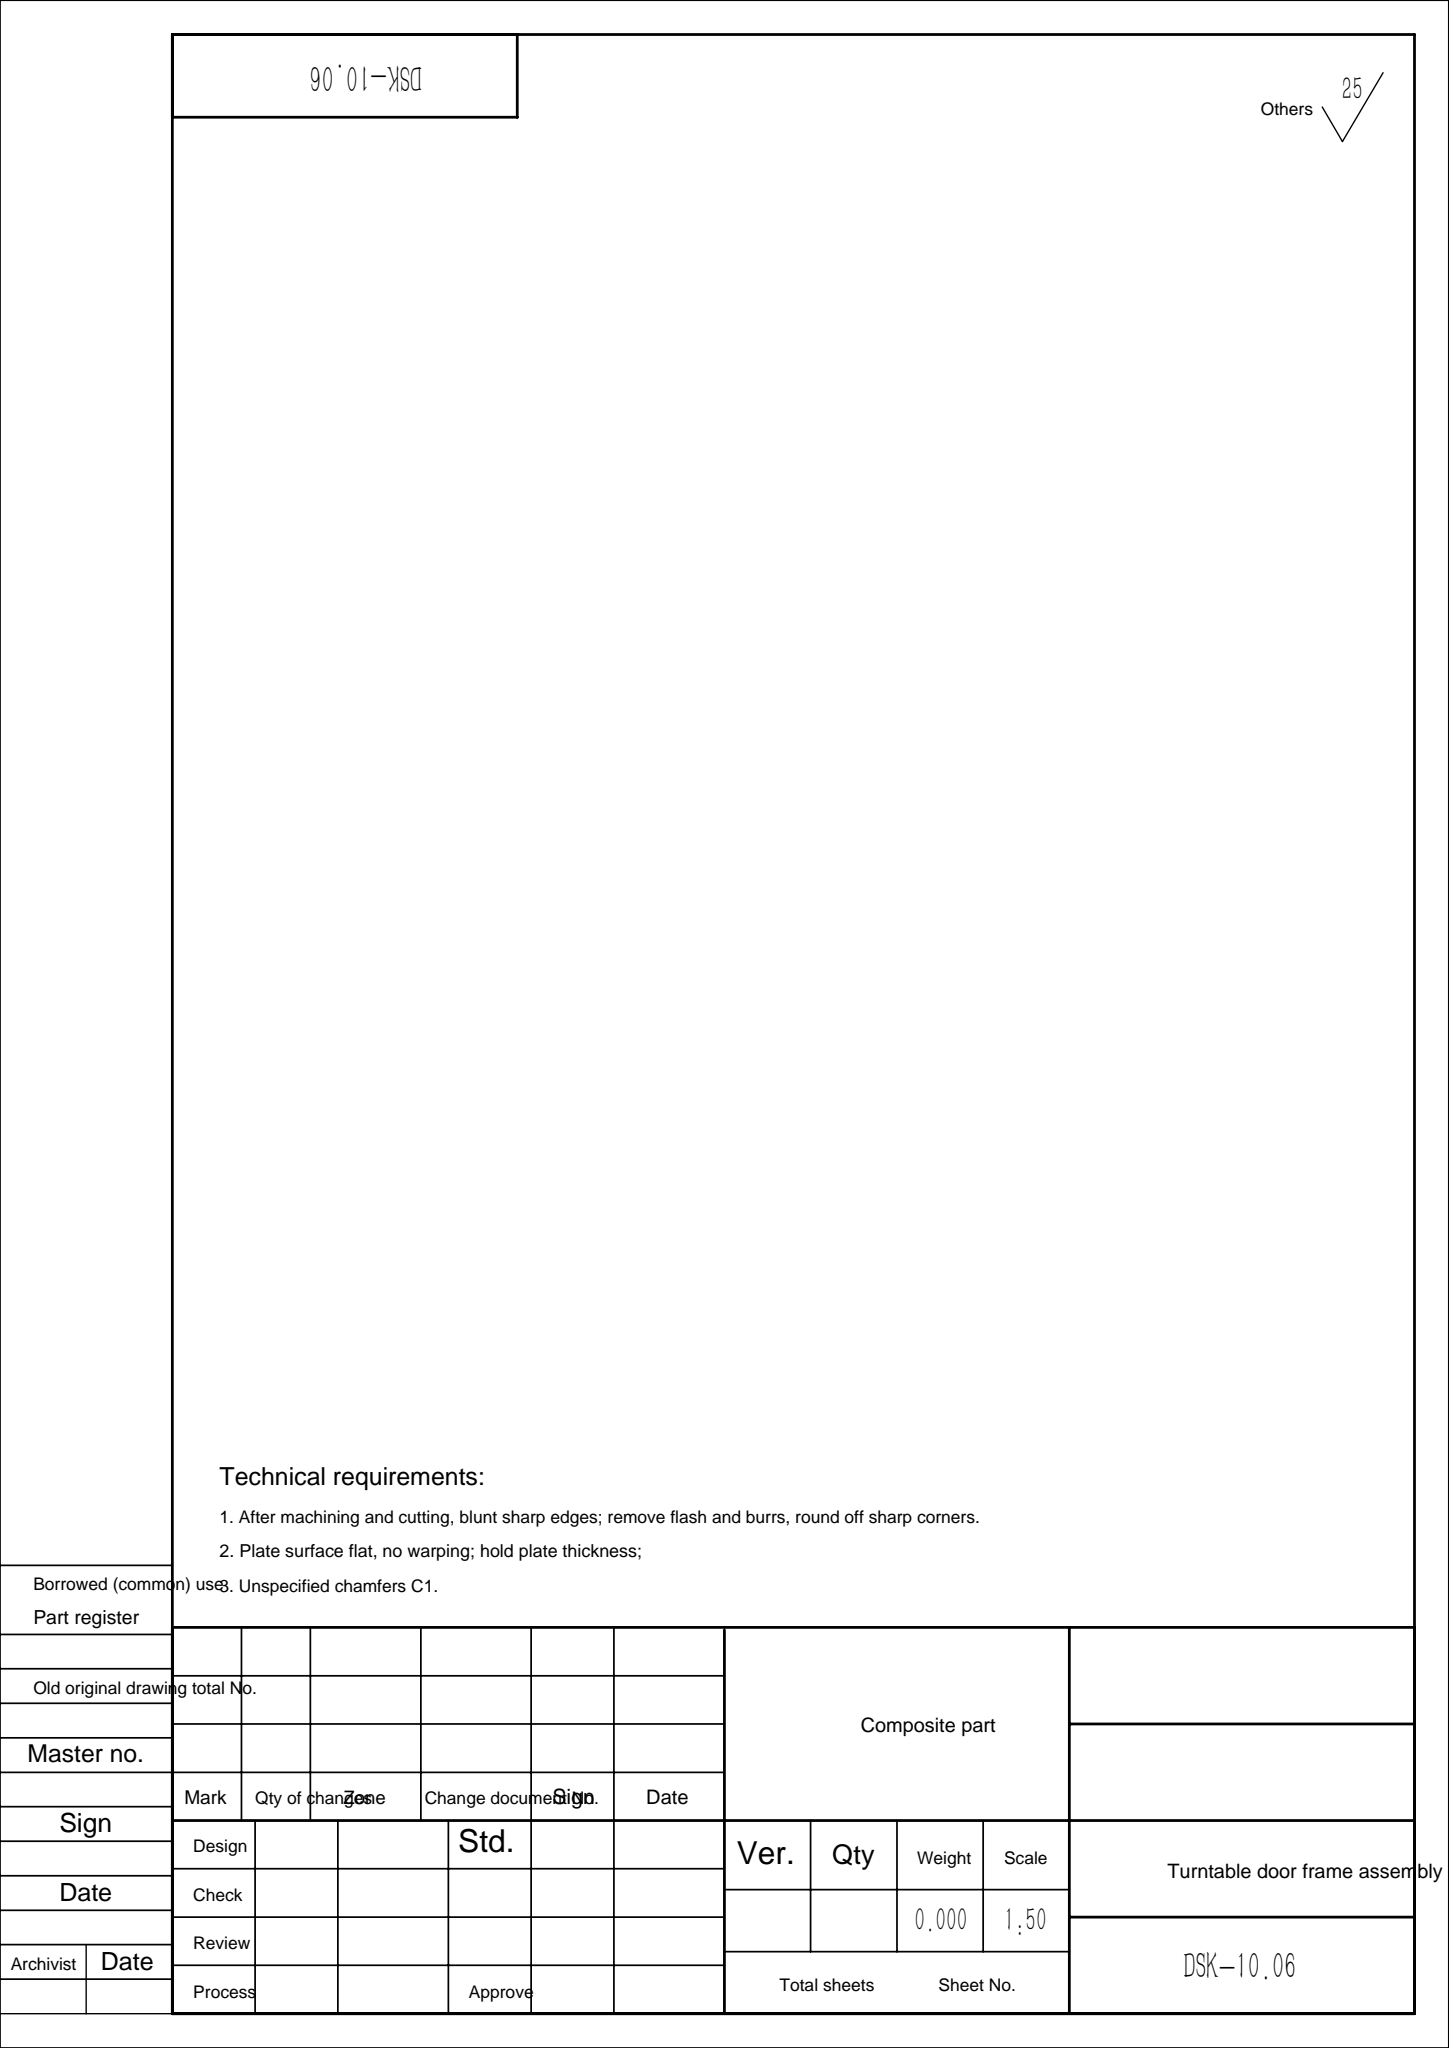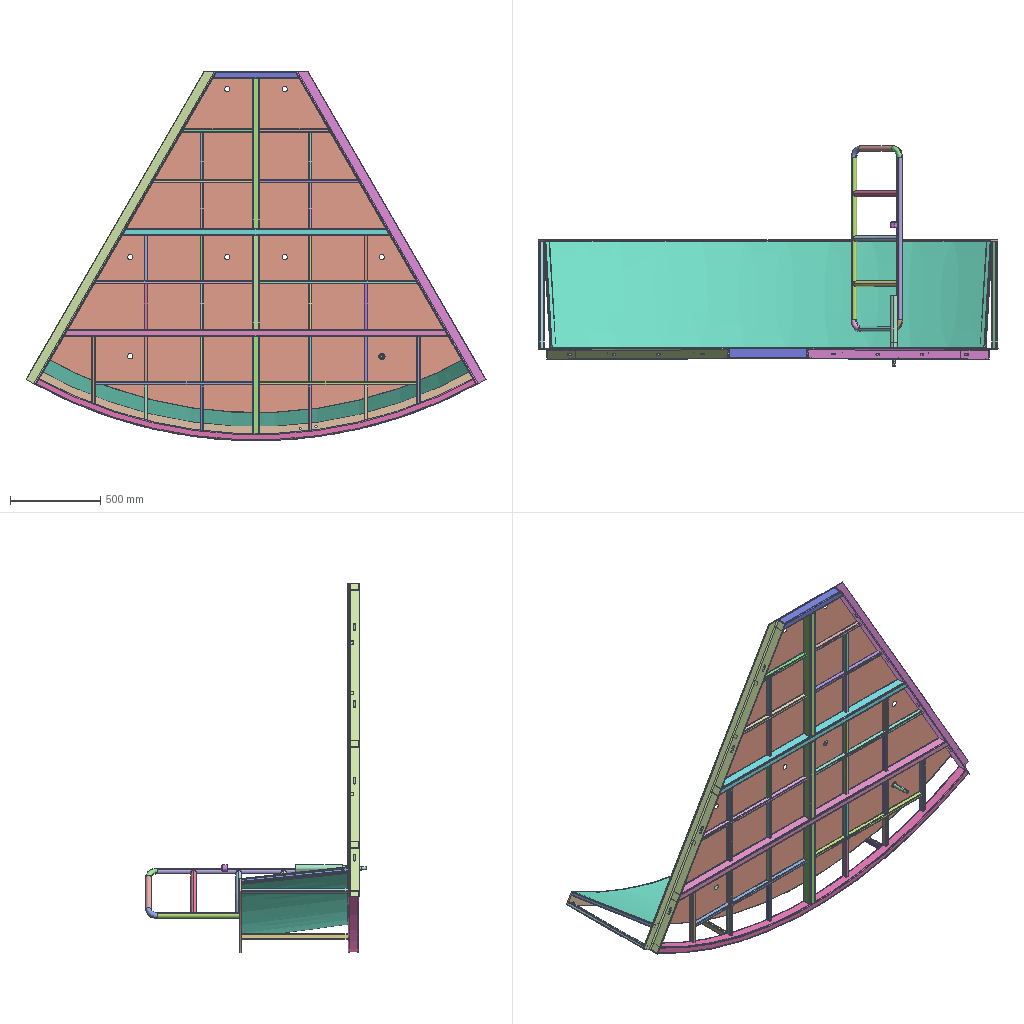Assembly | SolidWorks | 8 different items | 8 placed | box 2550 x 1224 x 2050 mm
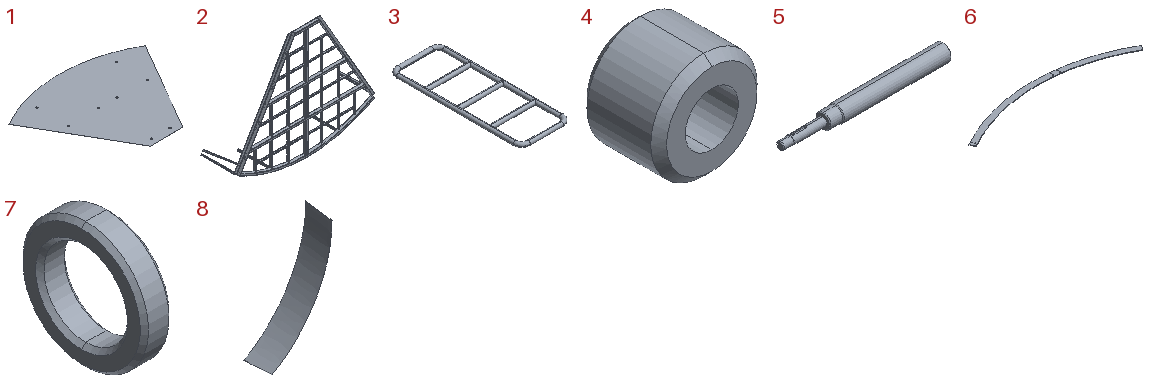Parts list (item | quantity | size | volume | features):
1 | x1 | 2393 x 1893 x 1 mm | 2848544 mm3 | features FlatPattern 1, HoleWzd 1, SMBaseFlange 1, SheetMetal 1
2 | x1 | 2550 x 655 x 2050 mm | 9987887 mm3 | features WeldCornerFeat 14, WeldMemberFeat 6, ICE 2, MirrorSolid 1, WeldmentFeature 1
3 | x1 | 387 x 1032 x 32 mm | 682567 mm3 | features WeldMemberFeat 1, WeldmentFeature 1
4 | x1 | 40 x 30 x 40 mm | 27200 mm3 | features Chamfer 1, Extrusion 1
5 | x1 | 393 x 40 x 40 mm | 386098 mm3 | features ICE 2, Chamfer 1, Revolution 1
6 | x1 | 2550 x 410.917 x 8 mm | 1676789 mm3 | features Extrusion 1, HoleWzd 1
7 | x1 | 6.9 x 30 x 30 mm | 2553 mm3 | features Chamfer 1, Extrusion 1
8 | x1 | 1273 x 598.126 x 2139 mm | 1534665 mm3 | features FlatPattern 1, ICE 1, LoftedBend 1, SheetMetal 1
Mates (type | each side: item.copy, entity, surface, feature):
Tangent | 3.1 face cylinder Gb/t 6728—2002 Round Tube 32 × 2-example.com(1) | 5.1 face cylinder Revolve1
DistanceDim | 4.1 face plane Boss-Extrude1 | 5.1 face plane Revolve1
Concentric | 4.1 face cylinder Boss-Extrude1 | 5.1 face cylinder Revolve1
Coincident | 1.1 face plane Base-Flange1 | 2.1 face plane Cold-formed hollow rectangular steel for structures (gb t6728-2002) 60×40×3(1) | 2 times
Coincident | 2.1 face plane Hot-rolled equal-leg angle steel (gb t9787-1988) 63×6(1) | 8.1 plane
Coincident | 2.1 face plane Cold-formed hollow rectangular steel for structures (gb t6728-2002) 30×20×2(2) | 8.1 face plane Cut-Extrude2
Concentric | 5.1 face cylinder Revolve1 | 1.1 face cylinder Ø30 Diameter Hole1
Coincident | 5.1 face plane Revolve1 | 1.1 face plane Base-Flange1
Concentric | 2.1 face cylinder Cold-formed hollow rectangular steel for structures (gb t6728-2002) 60×40×3(1) | 6.1 face cylinder Boss-Extrude1
Coincident | 2.1 face plane Trim/Extend18 | 6.1 face plane Boss-Extrude1
Parallel | 2.1 face plane Mirror1 | 6.1 face plane Boss-Extrude1
Concentric | 4.1 face cylinder Boss-Extrude1 | 7.1 face cylinder Boss-Extrude1
Coincident | 4.1 face plane Boss-Extrude1 | 7.1 face plane Boss-Extrude1
Coincident | 1.1 face plane Base-Flange1 | 2.1 face plane Hot-rolled equal-leg angle steel (gb t9787-1988) 63×6(1)
Coordinate | 2.1 select_type:25 | assembly select_type:11
Coincident | 2.1 face plane Mirror1 | 8.1 face plane Freeform Bend1